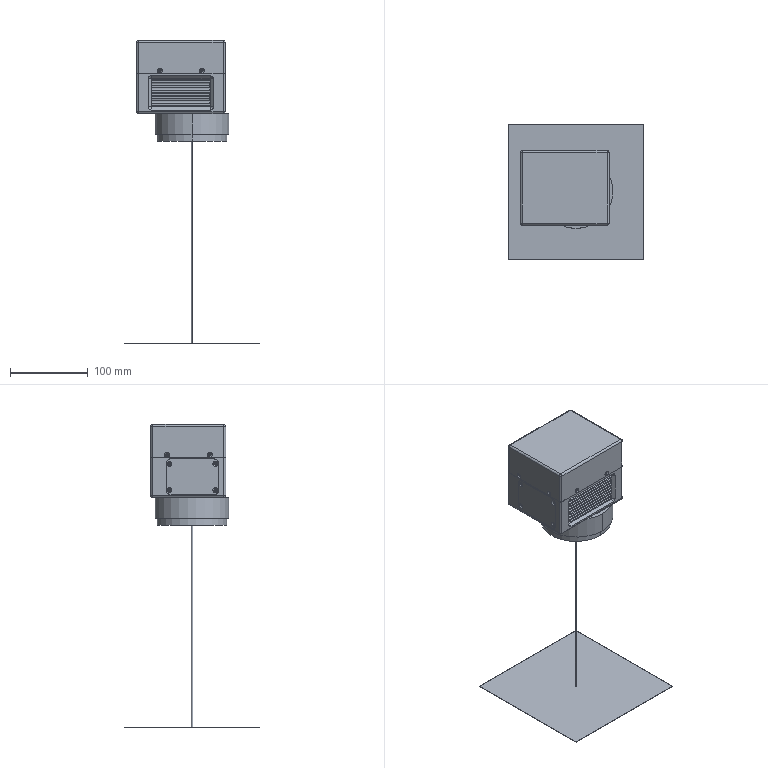Part | SolidWorks | features CompositeCurve 19 | 11 solids | 649 faces | box 175 x 175 x 390 mm | volume 804489 mm3 | cylinder 290 | plane 254 | cone 88 | spline 9 | sphere 8 | commonest cylinder face diameters 2.5 x30 5 x26 3.5 x24 12 x24 8 x22 3.3 x20